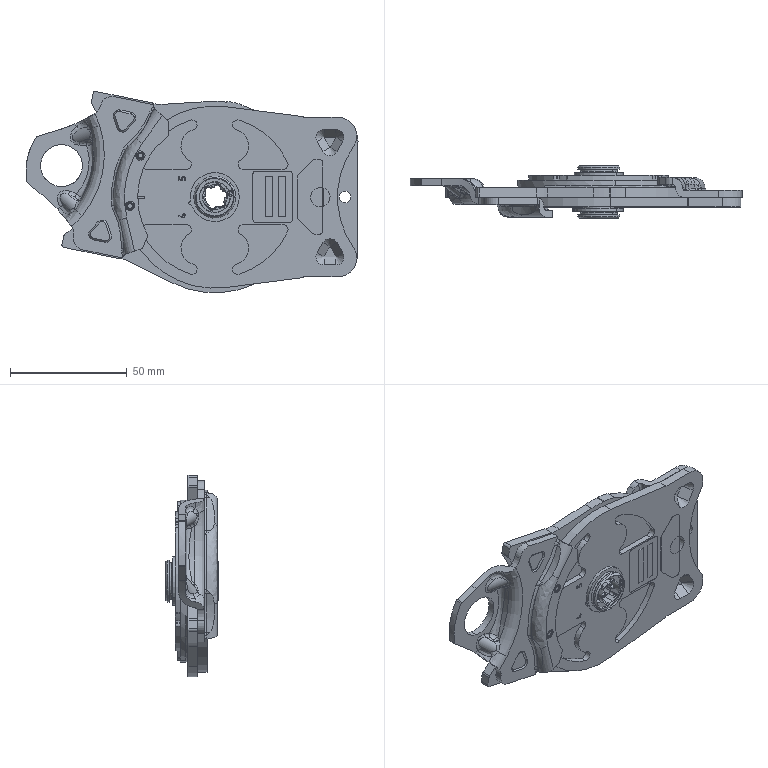Part | NX | features BREP 9 | 9 solids | 1236 faces | box 142.204 x 22.65 x 86.299 mm | volume 82065 mm3 | cylinder 440 | plane 365 | spline 250 | cone 94 | torus 71 | sphere 16 | commonest cylinder face diameters 0.3 x89 0.6 x66 1 x33 2 x25 3 x16 4 x16